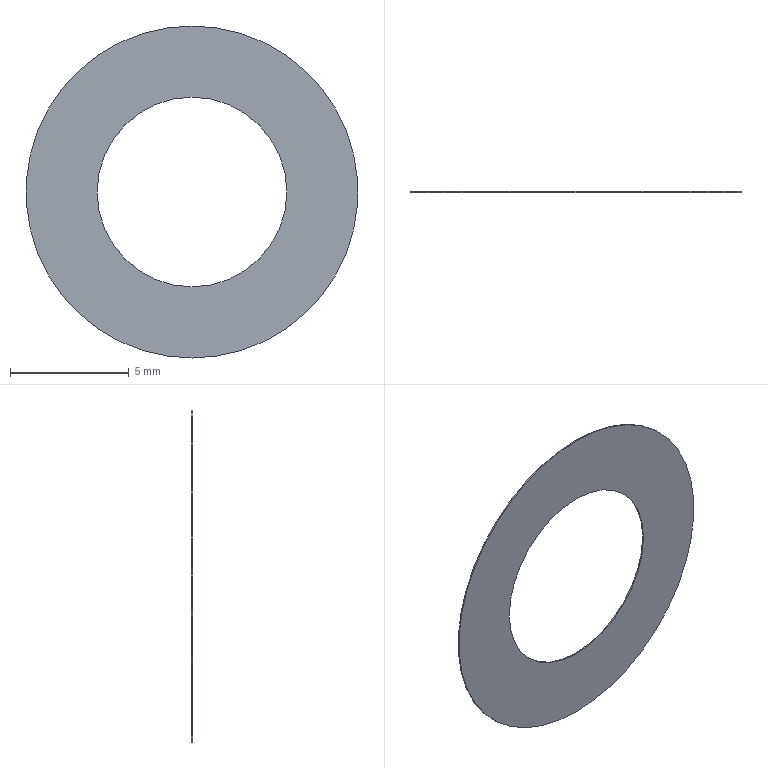Part | SolidWorks | features Extrusion 1 | 1 solid | 6 faces | box 14 x 0.05 x 14 mm | volume 5.184 mm3 | cylinder 4 | plane 2 | commonest cylinder face diameters 8 x2 14 x2
STEP:
#1=CARTESIAN_POINT('',(0.,0.05,-4.));
#2=VERTEX_POINT('',#1);
#3=CARTESIAN_POINT('',(0.,0.05,4.));
#4=VERTEX_POINT('',#3);
#5=CARTESIAN_POINT('',(0.,0.05,0.));
#6=DIRECTION('',(0.,1.,0.));
#7=DIRECTION('',(0.,0.,1.));
#8=AXIS2_PLACEMENT_3D('',#5,#6,#7);
#9=CIRCLE('',#8,4.);
#10=EDGE_CURVE('',#2,#4,#9,.T.);
#11=ORIENTED_EDGE('',*,*,#10,.T.);
#12=CARTESIAN_POINT('',(0.,0.,4.));
#13=VERTEX_POINT('',#12);
#14=CARTESIAN_POINT('',(0.,0.05,4.));
#15=DIRECTION('',(0.,-1.,0.));
#16=VECTOR('',#15,1000.);
#17=LINE('',#14,#16);
#18=EDGE_CURVE('',#4,#13,#17,.T.);
#19=ORIENTED_EDGE('',*,*,#18,.T.);
#20=CARTESIAN_POINT('',(0.,0.,-4.));
#21=VERTEX_POINT('',#20);
#22=CARTESIAN_POINT('',(0.,0.,0.));
#23=DIRECTION('',(0.,1.,0.));
#24=DIRECTION('',(0.,0.,1.));
#25=AXIS2_PLACEMENT_3D('',#22,#23,#24);
#26=CIRCLE('',#25,4.);
#27=EDGE_CURVE('',#21,#13,#26,.T.);
#28=ORIENTED_EDGE('',*,*,#27,.F.);
#29=CARTESIAN_POINT('',(0.,0.05,-4.));
#30=DIRECTION('',(0.,-1.,0.));
#31=VECTOR('',#30,1000.);
#32=LINE('',#29,#31);
#33=EDGE_CURVE('',#2,#21,#32,.T.);
#34=ORIENTED_EDGE('',*,*,#33,.F.);
#35=EDGE_LOOP('',(#11,#19,#28,#34));
#36=FACE_OUTER_BOUND('',#35,.T.);
#37=CARTESIAN_POINT('',(0.,0.05,0.));
#38=DIRECTION('',(0.,-1.,0.));
#39=DIRECTION('',(0.,0.,-1.));
#40=AXIS2_PLACEMENT_3D('',#37,#38,#39);
#41=CYLINDRICAL_SURFACE('',#40,4.);
#42=ADVANCED_FACE('',(#36),#41,.F.);
#43=CARTESIAN_POINT('',(0.,0.05,7.));
#44=VERTEX_POINT('',#43);
#45=CARTESIAN_POINT('',(0.,0.05,-7.));
#46=VERTEX_POINT('',#45);
#47=CARTESIAN_POINT('',(0.,0.05,0.));
#48=DIRECTION('',(0.,1.,0.));
#49=DIRECTION('',(0.,0.,1.));
#50=AXIS2_PLACEMENT_3D('',#47,#48,#49);
#51=CIRCLE('',#50,7.);
#52=EDGE_CURVE('',#44,#46,#51,.T.);
#53=ORIENTED_EDGE('',*,*,#52,.F.);
#54=CARTESIAN_POINT('',(0.,0.,7.));
#55=VERTEX_POINT('',#54);
#56=CARTESIAN_POINT('',(0.,0.05,7.));
#57=DIRECTION('',(0.,-1.,0.));
#58=VECTOR('',#57,1000.);
#59=LINE('',#56,#58);
#60=EDGE_CURVE('',#44,#55,#59,.T.);
#61=ORIENTED_EDGE('',*,*,#60,.T.);
#62=CARTESIAN_POINT('',(0.,0.,-7.));
#63=VERTEX_POINT('',#62);
#64=CARTESIAN_POINT('',(0.,0.,0.));
#65=DIRECTION('',(0.,1.,0.));
#66=DIRECTION('',(0.,0.,1.));
#67=AXIS2_PLACEMENT_3D('',#64,#65,#66);
#68=CIRCLE('',#67,7.);
#69=EDGE_CURVE('',#55,#63,#68,.T.);
#70=ORIENTED_EDGE('',*,*,#69,.T.);
#71=CARTESIAN_POINT('',(0.,0.05,-7.));
#72=DIRECTION('',(0.,-1.,0.));
#73=VECTOR('',#72,1000.);
#74=LINE('',#71,#73);
#75=EDGE_CURVE('',#46,#63,#74,.T.);
#76=ORIENTED_EDGE('',*,*,#75,.F.);
#77=EDGE_LOOP('',(#53,#61,#70,#76));
#78=FACE_OUTER_BOUND('',#77,.T.);
#79=CARTESIAN_POINT('',(0.,0.05,0.));
#80=DIRECTION('',(0.,-1.,0.));
#81=DIRECTION('',(0.,0.,-1.));
#82=AXIS2_PLACEMENT_3D('',#79,#80,#81);
#83=CYLINDRICAL_SURFACE('',#82,7.);
#84=ADVANCED_FACE('',(#78),#83,.T.);
#85=CARTESIAN_POINT('',(0.,0.05,0.));
#86=DIRECTION('',(0.,1.,0.));
#87=DIRECTION('',(0.,0.,1.));
#88=AXIS2_PLACEMENT_3D('',#85,#86,#87);
#89=CIRCLE('',#88,7.);
#90=EDGE_CURVE('',#46,#44,#89,.T.);
#91=ORIENTED_EDGE('',*,*,#90,.T.);
#92=ORIENTED_EDGE('',*,*,#52,.T.);
#93=EDGE_LOOP('',(#91,#92));
#94=FACE_OUTER_BOUND('',#93,.T.);
#95=ORIENTED_EDGE('',*,*,#10,.F.);
#96=CARTESIAN_POINT('',(0.,0.05,0.));
#97=DIRECTION('',(0.,1.,0.));
#98=DIRECTION('',(0.,0.,1.));
#99=AXIS2_PLACEMENT_3D('',#96,#97,#98);
#100=CIRCLE('',#99,4.);
#101=EDGE_CURVE('',#4,#2,#100,.T.);
#102=ORIENTED_EDGE('',*,*,#101,.F.);
#103=EDGE_LOOP('',(#95,#102));
#104=FACE_BOUND('',#103,.T.);
#105=CARTESIAN_POINT('',(0.,0.05,0.));
#106=DIRECTION('',(0.,1.,0.));
#107=DIRECTION('',(0.,0.,1.));
#108=AXIS2_PLACEMENT_3D('',#105,#106,#107);
#109=PLANE('',#108);
#110=ADVANCED_FACE('',(#94,#104),#109,.T.);
#111=CARTESIAN_POINT('',(0.,0.,0.));
#112=DIRECTION('',(0.,1.,0.));
#113=DIRECTION('',(0.,0.,1.));
#114=AXIS2_PLACEMENT_3D('',#111,#112,#113);
#115=CIRCLE('',#114,7.);
#116=EDGE_CURVE('',#63,#55,#115,.T.);
#117=ORIENTED_EDGE('',*,*,#116,.F.);
#118=ORIENTED_EDGE('',*,*,#69,.F.);
#119=EDGE_LOOP('',(#117,#118));
#120=FACE_OUTER_BOUND('',#119,.T.);
#121=ORIENTED_EDGE('',*,*,#27,.T.);
#122=CARTESIAN_POINT('',(0.,0.,0.));
#123=DIRECTION('',(0.,1.,0.));
#124=DIRECTION('',(0.,0.,1.));
#125=AXIS2_PLACEMENT_3D('',#122,#123,#124);
#126=CIRCLE('',#125,4.);
#127=EDGE_CURVE('',#13,#21,#126,.T.);
#128=ORIENTED_EDGE('',*,*,#127,.T.);
#129=EDGE_LOOP('',(#121,#128));
#130=FACE_BOUND('',#129,.T.);
#131=CARTESIAN_POINT('',(0.,0.,0.));
#132=DIRECTION('',(0.,1.,0.));
#133=DIRECTION('',(0.,0.,1.));
#134=AXIS2_PLACEMENT_3D('',#131,#132,#133);
#135=PLANE('',#134);
#136=ADVANCED_FACE('',(#120,#130),#135,.F.);
#137=ORIENTED_EDGE('',*,*,#60,.F.);
#138=ORIENTED_EDGE('',*,*,#90,.F.);
#139=ORIENTED_EDGE('',*,*,#75,.T.);
#140=ORIENTED_EDGE('',*,*,#116,.T.);
#141=EDGE_LOOP('',(#137,#138,#139,#140));
#142=FACE_OUTER_BOUND('',#141,.T.);
#143=CARTESIAN_POINT('',(0.,0.05,0.));
#144=DIRECTION('',(0.,-1.,0.));
#145=DIRECTION('',(0.,0.,-1.));
#146=AXIS2_PLACEMENT_3D('',#143,#144,#145);
#147=CYLINDRICAL_SURFACE('',#146,7.);
#148=ADVANCED_FACE('',(#142),#147,.T.);
#149=ORIENTED_EDGE('',*,*,#18,.F.);
#150=ORIENTED_EDGE('',*,*,#101,.T.);
#151=ORIENTED_EDGE('',*,*,#33,.T.);
#152=ORIENTED_EDGE('',*,*,#127,.F.);
#153=EDGE_LOOP('',(#149,#150,#151,#152));
#154=FACE_OUTER_BOUND('',#153,.T.);
#155=CARTESIAN_POINT('',(0.,0.05,0.));
#156=DIRECTION('',(0.,-1.,0.));
#157=DIRECTION('',(0.,0.,-1.));
#158=AXIS2_PLACEMENT_3D('',#155,#156,#157);
#159=CYLINDRICAL_SURFACE('',#158,4.);
#160=ADVANCED_FACE('',(#154),#159,.F.);
#161=CLOSED_SHELL('',(#42,#84,#110,#136,#148,#160));
#162=MANIFOLD_SOLID_BREP('',#161);
#163=CARTESIAN_POINT('',(0.,0.,0.));
#164=DIRECTION('',(0.,0.,1.));
#165=DIRECTION('',(1.,0.,0.));
#166=AXIS2_PLACEMENT_3D('',#163,#164,#165);
#167=(LENGTH_UNIT()NAMED_UNIT(*)SI_UNIT(.MILLI.,.METRE.));
#168=UNCERTAINTY_MEASURE_WITH_UNIT(LENGTH_MEASURE(0.00001),#167,'','');
#169=(NAMED_UNIT(*)PLANE_ANGLE_UNIT()SI_UNIT($,.RADIAN.));
#170=(NAMED_UNIT(*)SI_UNIT($,.STERADIAN.)SOLID_ANGLE_UNIT());
#171=(GEOMETRIC_REPRESENTATION_CONTEXT(3)GLOBAL_UNCERTAINTY_ASSIGNED_CONTEXT((#168))GLOBAL_UNIT_ASSIGNED_CONTEXT((#167,#169,#170))REPRESENTATION_CONTEXT('',''));
#172=ADVANCED_BREP_SHAPE_REPRESENTATION('',(#162,#166),#171);